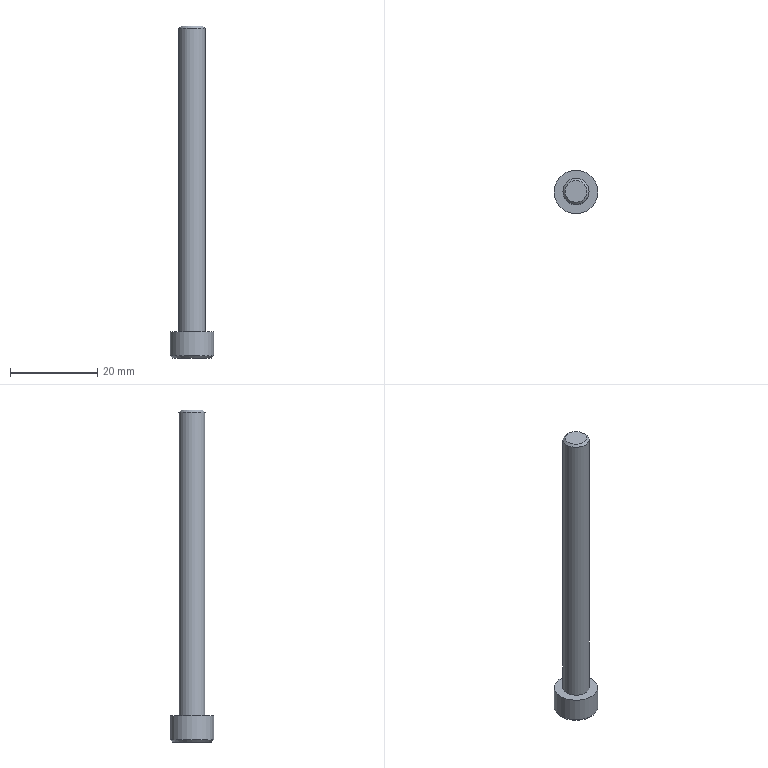Part | STEP file | M6.00-80.00 | 1 solid | 14 faces | box 10 x 10 x 76 mm | volume 2379 mm3 | plane 10 | cylinder 2 | cone 2 | commonest cylinder face diameters 6 x1 10 x1